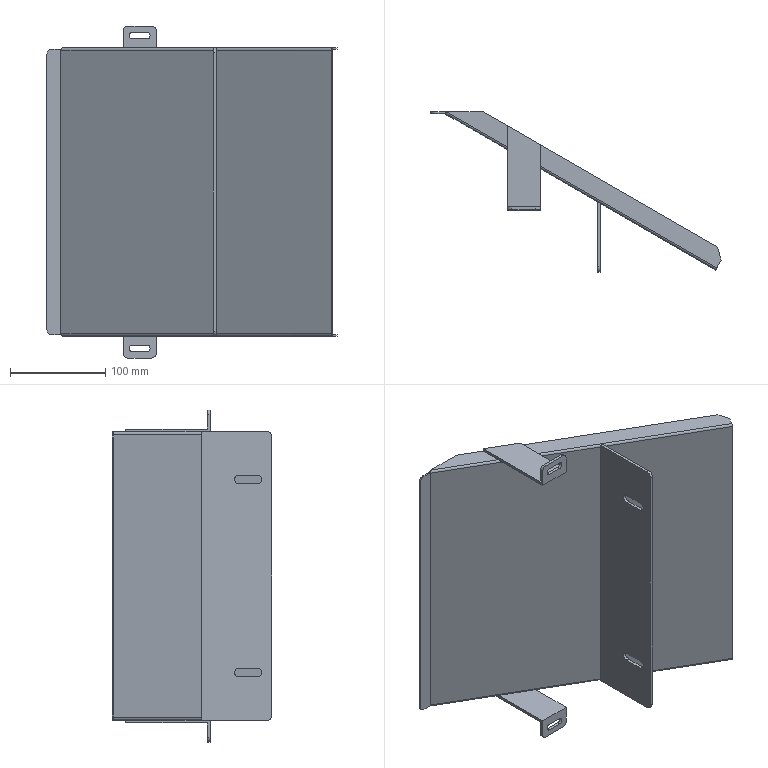Part | STEP file | PN_0039 | 4 solids | 82 faces | box 305 x 168 x 349 mm | volume 258678 mm3 | plane 58 | cylinder 22 | spline 2 | commonest cylinder face diameters 10 x8 7 x4 9 x4 1.473 x3 4.473 x3